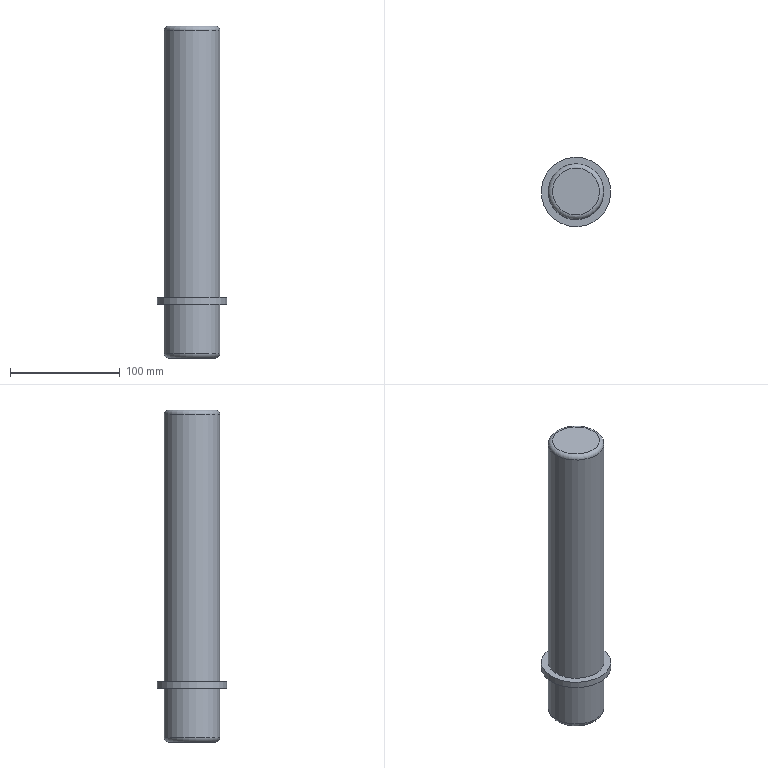Part | STEP file | 1_id1266_x_t | 1 solid | 12 faces | box 63.5 x 63.5 x 303.213 mm | volume 619621 mm3 | cylinder 4 | plane 4 | torus 2 | cone 2 | commonest cylinder face diameters 50.8 x2 4.2 x1 63.5 x1
STEP:
#1=CARTESIAN_POINT('',(0.,0.,0.));
#2=DIRECTION('',(0.,0.,1.));
#3=DIRECTION('',(1.,0.,0.));
#4=AXIS2_PLACEMENT_3D('',#1,#2,#3);
#5=CARTESIAN_POINT('',(-35.188,-151.958,160.));
#6=VERTEX_POINT('',#5);
#7=CARTESIAN_POINT('',(-2.535,-113.042,160.));
#8=VERTEX_POINT('',#7);
#9=CARTESIAN_POINT('',(-18.862,-132.5,160.));
#10=DIRECTION('',(0.,0.,1.));
#11=DIRECTION('',(0.6428,0.766,0.));
#12=AXIS2_PLACEMENT_3D('',#9,#10,#11);
#13=CIRCLE('',#12,25.4);
#14=CARTESIAN_POINT('',(-18.862,-132.5,34.6));
#15=DIRECTION('',(0.,0.,1.));
#16=DIRECTION('',(-0.6428,-0.766,0.));
#17=AXIS2_PLACEMENT_3D('',#14,#15,#16);
#18=CYLINDRICAL_SURFACE('',#17,25.4);
#19=CARTESIAN_POINT('',(-3.142,125.4));
#20=DIRECTION('',(1.,0.));
#21=VECTOR('',#20,1.);
#22=LINE('',#19,#21);
#23=(GEOMETRIC_REPRESENTATION_CONTEXT(2)PARAMETRIC_REPRESENTATION_CONTEXT()REPRESENTATION_CONTEXT('',''));
#24=DEFINITIONAL_REPRESENTATION('',(#22),#23);
#25=PCURVE('',#18,#24);
#26=CARTESIAN_POINT('',(-18.862,-132.5,160.));
#27=DIRECTION('',(0.,0.,1.));
#28=DIRECTION('',(0.6428,0.766,0.));
#29=AXIS2_PLACEMENT_3D('',#26,#27,#28);
#30=TOROIDAL_SURFACE('',#29,21.4,4.);
#31=CARTESIAN_POINT('',(0.,6.283));
#32=DIRECTION('',(1.,0.));
#33=VECTOR('',#32,1.);
#34=LINE('',#31,#33);
#35=(GEOMETRIC_REPRESENTATION_CONTEXT(2)PARAMETRIC_REPRESENTATION_CONTEXT()REPRESENTATION_CONTEXT('',''));
#36=DEFINITIONAL_REPRESENTATION('',(#34),#35);
#37=PCURVE('',#30,#36);
#38=SURFACE_CURVE('',#13,(#25,#37),.PCURVE_S1.);
#39=EDGE_CURVE('',#6,#8,#38,.T.);
#40=ORIENTED_EDGE('',*,*,#39,.F.);
#41=CARTESIAN_POINT('',(-35.188,-151.958,-84.));
#42=VERTEX_POINT('',#41);
#43=CARTESIAN_POINT('',(-35.188,-151.958,-84.));
#44=CARTESIAN_POINT('',(-35.188,-151.958,160.));
#45=B_SPLINE_CURVE_WITH_KNOTS('',1,(#43,#44),.UNSPECIFIED.,.F.,.F.,(2,2),(-118.6,125.4),.PIECEWISE_BEZIER_KNOTS.);
#46=CARTESIAN_POINT('',(0.,0.));
#47=DIRECTION('',(0.,1.));
#48=VECTOR('',#47,1.);
#49=LINE('',#46,#48);
#50=(GEOMETRIC_REPRESENTATION_CONTEXT(2)PARAMETRIC_REPRESENTATION_CONTEXT()REPRESENTATION_CONTEXT('',''));
#51=DEFINITIONAL_REPRESENTATION('',(#49),#50);
#52=PCURVE('',#18,#51);
#53=CARTESIAN_POINT('',(6.283,0.));
#54=DIRECTION('',(0.,1.));
#55=VECTOR('',#54,1.);
#56=LINE('',#53,#55);
#57=(GEOMETRIC_REPRESENTATION_CONTEXT(2)PARAMETRIC_REPRESENTATION_CONTEXT()REPRESENTATION_CONTEXT('',''));
#58=DEFINITIONAL_REPRESENTATION('',(#56),#57);
#59=PCURVE('',#18,#58);
#60=SEAM_CURVE('',#45,(#52,#59),.PCURVE_S1.);
#61=EDGE_CURVE('',#42,#6,#60,.T.);
#62=ORIENTED_EDGE('',*,*,#61,.F.);
#63=CARTESIAN_POINT('',(-18.862,-132.5,-84.));
#64=DIRECTION('',(0.,0.,-1.));
#65=DIRECTION('',(-0.6428,-0.766,0.));
#66=AXIS2_PLACEMENT_3D('',#63,#64,#65);
#67=CIRCLE('',#66,25.4);
#68=CARTESIAN_POINT('',(6.283,-118.6));
#69=DIRECTION('',(-1.,0.));
#70=VECTOR('',#69,1.);
#71=LINE('',#68,#70);
#72=(GEOMETRIC_REPRESENTATION_CONTEXT(2)PARAMETRIC_REPRESENTATION_CONTEXT()REPRESENTATION_CONTEXT('',''));
#73=DEFINITIONAL_REPRESENTATION('',(#71),#72);
#74=PCURVE('',#18,#73);
#75=CARTESIAN_POINT('',(-18.862,-132.5,-84.));
#76=DIRECTION('',(0.,0.,1.));
#77=DIRECTION('',(-0.6428,-0.766,0.));
#78=AXIS2_PLACEMENT_3D('',#75,#76,#77);
#79=PLANE('',#78);
#80=CARTESIAN_POINT('',(25.4,0.));
#81=CARTESIAN_POINT('',(25.4,-43.994));
#82=CARTESIAN_POINT('',(-12.7,-21.997));
#83=CARTESIAN_POINT('',(-50.8,0.));
#84=CARTESIAN_POINT('',(-12.7,21.997));
#85=CARTESIAN_POINT('',(25.4,43.994));
#86=CARTESIAN_POINT('',(25.4,0.));
#87=(BOUNDED_CURVE()B_SPLINE_CURVE(2,(#80,#81,#82,#83,#84,#85,#86),.UNSPECIFIED.,.T.,.F.)B_SPLINE_CURVE_WITH_KNOTS((1,2,2,2,2,1),(-2.094,0.,2.094,4.189,6.283,8.378),.UNSPECIFIED.)CURVE()GEOMETRIC_REPRESENTATION_ITEM()RATIONAL_B_SPLINE_CURVE((1.,0.5,1.,0.5,1.,0.5,1.))REPRESENTATION_ITEM(''));
#88=(GEOMETRIC_REPRESENTATION_CONTEXT(2)PARAMETRIC_REPRESENTATION_CONTEXT()REPRESENTATION_CONTEXT('',''));
#89=DEFINITIONAL_REPRESENTATION('',(#87),#88);
#90=PCURVE('',#79,#89);
#91=SURFACE_CURVE('',#67,(#74,#90),.PCURVE_S1.);
#92=EDGE_CURVE('',#42,#42,#91,.T.);
#93=ORIENTED_EDGE('',*,*,#92,.F.);
#94=ORIENTED_EDGE('',*,*,#61,.T.);
#95=CARTESIAN_POINT('',(-18.862,-132.5,160.));
#96=DIRECTION('',(0.,0.,1.));
#97=DIRECTION('',(0.6428,0.766,0.));
#98=AXIS2_PLACEMENT_3D('',#95,#96,#97);
#99=CIRCLE('',#98,25.4);
#100=CARTESIAN_POINT('',(3.142,125.4));
#101=DIRECTION('',(1.,0.));
#102=VECTOR('',#101,1.);
#103=LINE('',#100,#102);
#104=(GEOMETRIC_REPRESENTATION_CONTEXT(2)PARAMETRIC_REPRESENTATION_CONTEXT()REPRESENTATION_CONTEXT('',''));
#105=DEFINITIONAL_REPRESENTATION('',(#103),#104);
#106=PCURVE('',#18,#105);
#107=CARTESIAN_POINT('',(0.,6.283));
#108=DIRECTION('',(1.,0.));
#109=VECTOR('',#108,1.);
#110=LINE('',#107,#109);
#111=(GEOMETRIC_REPRESENTATION_CONTEXT(2)PARAMETRIC_REPRESENTATION_CONTEXT()REPRESENTATION_CONTEXT('',''));
#112=DEFINITIONAL_REPRESENTATION('',(#110),#111);
#113=PCURVE('',#30,#112);
#114=SURFACE_CURVE('',#99,(#106,#113),.PCURVE_S1.);
#115=EDGE_CURVE('',#8,#6,#114,.T.);
#116=ORIENTED_EDGE('',*,*,#115,.F.);
#117=EDGE_LOOP('',(#40,#62,#93,#94,#116));
#118=FACE_BOUND('',#117,.T.);
#119=ADVANCED_FACE('',(#118),#18,.T.);
#120=CARTESIAN_POINT('',(-39.27,-156.822,-84.));
#121=VERTEX_POINT('',#120);
#122=CARTESIAN_POINT('',(-18.862,-132.5,-84.));
#123=DIRECTION('',(0.,0.,1.));
#124=DIRECTION('',(-0.6428,-0.766,0.));
#125=AXIS2_PLACEMENT_3D('',#122,#123,#124);
#126=CIRCLE('',#125,31.75);
#127=CARTESIAN_POINT('',(0.,0.));
#128=DIRECTION('',(1.,0.));
#129=AXIS2_PLACEMENT_2D('',#127,#128);
#130=CIRCLE('',#129,31.75);
#131=(GEOMETRIC_REPRESENTATION_CONTEXT(2)PARAMETRIC_REPRESENTATION_CONTEXT()REPRESENTATION_CONTEXT('',''));
#132=DEFINITIONAL_REPRESENTATION('',(#130),#131);
#133=PCURVE('',#79,#132);
#134=CARTESIAN_POINT('',(-18.862,-132.5,-84.));
#135=DIRECTION('',(0.,0.,1.));
#136=DIRECTION('',(-0.6428,-0.766,0.));
#137=AXIS2_PLACEMENT_3D('',#134,#135,#136);
#138=CYLINDRICAL_SURFACE('',#137,31.75);
#139=CARTESIAN_POINT('',(0.,0.));
#140=DIRECTION('',(1.,0.));
#141=VECTOR('',#140,1.);
#142=LINE('',#139,#141);
#143=(GEOMETRIC_REPRESENTATION_CONTEXT(2)PARAMETRIC_REPRESENTATION_CONTEXT()REPRESENTATION_CONTEXT('',''));
#144=DEFINITIONAL_REPRESENTATION('',(#142),#143);
#145=PCURVE('',#138,#144);
#146=SURFACE_CURVE('',#126,(#133,#145),.PCURVE_S1.);
#147=EDGE_CURVE('',#121,#121,#146,.T.);
#148=ORIENTED_EDGE('',*,*,#147,.T.);
#149=EDGE_LOOP('',(#148));
#150=FACE_BOUND('',#149,.T.);
#151=ORIENTED_EDGE('',*,*,#92,.T.);
#152=EDGE_LOOP('',(#151));
#153=FACE_BOUND('',#152,.T.);
#154=ADVANCED_FACE('',(#150,#153),#79,.T.);
#155=ORIENTED_EDGE('',*,*,#147,.F.);
#156=CARTESIAN_POINT('',(-39.27,-156.822,-90.));
#157=VERTEX_POINT('',#156);
#158=CARTESIAN_POINT('',(-39.27,-156.822,-90.));
#159=CARTESIAN_POINT('',(-39.27,-156.822,-84.));
#160=B_SPLINE_CURVE_WITH_KNOTS('',1,(#158,#159),.UNSPECIFIED.,.F.,.F.,(2,2),(-6.,0.),.PIECEWISE_BEZIER_KNOTS.);
#161=CARTESIAN_POINT('',(0.,0.));
#162=DIRECTION('',(0.,1.));
#163=VECTOR('',#162,1.);
#164=LINE('',#161,#163);
#165=(GEOMETRIC_REPRESENTATION_CONTEXT(2)PARAMETRIC_REPRESENTATION_CONTEXT()REPRESENTATION_CONTEXT('',''));
#166=DEFINITIONAL_REPRESENTATION('',(#164),#165);
#167=PCURVE('',#138,#166);
#168=CARTESIAN_POINT('',(6.283,0.));
#169=DIRECTION('',(0.,1.));
#170=VECTOR('',#169,1.);
#171=LINE('',#168,#170);
#172=(GEOMETRIC_REPRESENTATION_CONTEXT(2)PARAMETRIC_REPRESENTATION_CONTEXT()REPRESENTATION_CONTEXT('',''));
#173=DEFINITIONAL_REPRESENTATION('',(#171),#172);
#174=PCURVE('',#138,#173);
#175=SEAM_CURVE('',#160,(#167,#174),.PCURVE_S1.);
#176=EDGE_CURVE('',#157,#121,#175,.T.);
#177=ORIENTED_EDGE('',*,*,#176,.F.);
#178=CARTESIAN_POINT('',(1.547,-108.178,-90.));
#179=VERTEX_POINT('',#178);
#180=CARTESIAN_POINT('',(-18.862,-132.5,-90.));
#181=DIRECTION('',(0.,0.,-1.));
#182=DIRECTION('',(0.6428,0.766,0.));
#183=AXIS2_PLACEMENT_3D('',#180,#181,#182);
#184=CIRCLE('',#183,31.75);
#185=CARTESIAN_POINT('',(3.142,-6.));
#186=DIRECTION('',(-1.,0.));
#187=VECTOR('',#186,1.);
#188=LINE('',#185,#187);
#189=(GEOMETRIC_REPRESENTATION_CONTEXT(2)PARAMETRIC_REPRESENTATION_CONTEXT()REPRESENTATION_CONTEXT('',''));
#190=DEFINITIONAL_REPRESENTATION('',(#188),#189);
#191=PCURVE('',#138,#190);
#192=CARTESIAN_POINT('',(-18.862,-132.5,-90.));
#193=DIRECTION('',(0.,0.,1.));
#194=DIRECTION('',(-0.6428,-0.766,0.));
#195=AXIS2_PLACEMENT_3D('',#192,#193,#194);
#196=PLANE('',#195);
#197=CARTESIAN_POINT('',(-31.75,0.));
#198=CARTESIAN_POINT('',(-31.75,54.993));
#199=CARTESIAN_POINT('',(15.875,27.496));
#200=CARTESIAN_POINT('',(63.5,0.));
#201=CARTESIAN_POINT('',(15.875,-27.496));
#202=CARTESIAN_POINT('',(-31.75,-54.993));
#203=CARTESIAN_POINT('',(-31.75,0.));
#204=(BOUNDED_CURVE()B_SPLINE_CURVE(2,(#197,#198,#199,#200,#201,#202,#203),.UNSPECIFIED.,.T.,.F.)B_SPLINE_CURVE_WITH_KNOTS((1,2,2,2,2,1),(-2.094,0.,2.094,4.189,6.283,8.378),.UNSPECIFIED.)CURVE()GEOMETRIC_REPRESENTATION_ITEM()RATIONAL_B_SPLINE_CURVE((1.,0.5,1.,0.5,1.,0.5,1.))REPRESENTATION_ITEM(''));
#205=(GEOMETRIC_REPRESENTATION_CONTEXT(2)PARAMETRIC_REPRESENTATION_CONTEXT()REPRESENTATION_CONTEXT('',''));
#206=DEFINITIONAL_REPRESENTATION('',(#204),#205);
#207=PCURVE('',#196,#206);
#208=SURFACE_CURVE('',#184,(#191,#207),.PCURVE_S1.);
#209=EDGE_CURVE('',#179,#157,#208,.T.);
#210=ORIENTED_EDGE('',*,*,#209,.F.);
#211=CARTESIAN_POINT('',(-18.862,-132.5,-90.));
#212=DIRECTION('',(0.,0.,-1.));
#213=DIRECTION('',(0.6428,0.766,0.));
#214=AXIS2_PLACEMENT_3D('',#211,#212,#213);
#215=CIRCLE('',#214,31.75);
#216=CARTESIAN_POINT('',(9.425,-6.));
#217=DIRECTION('',(-1.,0.));
#218=VECTOR('',#217,1.);
#219=LINE('',#216,#218);
#220=(GEOMETRIC_REPRESENTATION_CONTEXT(2)PARAMETRIC_REPRESENTATION_CONTEXT()REPRESENTATION_CONTEXT('',''));
#221=DEFINITIONAL_REPRESENTATION('',(#219),#220);
#222=PCURVE('',#138,#221);
#223=CARTESIAN_POINT('',(-31.75,0.));
#224=CARTESIAN_POINT('',(-31.75,54.993));
#225=CARTESIAN_POINT('',(15.875,27.496));
#226=CARTESIAN_POINT('',(63.5,0.));
#227=CARTESIAN_POINT('',(15.875,-27.496));
#228=CARTESIAN_POINT('',(-31.75,-54.993));
#229=CARTESIAN_POINT('',(-31.75,0.));
#230=(BOUNDED_CURVE()B_SPLINE_CURVE(2,(#223,#224,#225,#226,#227,#228,#229),.UNSPECIFIED.,.T.,.F.)B_SPLINE_CURVE_WITH_KNOTS((1,2,2,2,2,1),(-2.094,0.,2.094,4.189,6.283,8.378),.UNSPECIFIED.)CURVE()GEOMETRIC_REPRESENTATION_ITEM()RATIONAL_B_SPLINE_CURVE((1.,0.5,1.,0.5,1.,0.5,1.))REPRESENTATION_ITEM(''));
#231=(GEOMETRIC_REPRESENTATION_CONTEXT(2)PARAMETRIC_REPRESENTATION_CONTEXT()REPRESENTATION_CONTEXT('',''));
#232=DEFINITIONAL_REPRESENTATION('',(#230),#231);
#233=PCURVE('',#196,#232);
#234=SURFACE_CURVE('',#215,(#222,#233),.PCURVE_S1.);
#235=EDGE_CURVE('',#157,#179,#234,.T.);
#236=ORIENTED_EDGE('',*,*,#235,.F.);
#237=ORIENTED_EDGE('',*,*,#176,.T.);
#238=EDGE_LOOP('',(#155,#177,#210,#236,#237));
#239=FACE_BOUND('',#238,.T.);
#240=ADVANCED_FACE('',(#239),#138,.T.);
#241=ORIENTED_EDGE('',*,*,#209,.T.);
#242=ORIENTED_EDGE('',*,*,#235,.T.);
#243=EDGE_LOOP('',(#241,#242));
#244=FACE_BOUND('',#243,.T.);
#245=CARTESIAN_POINT('',(-35.188,-151.958,-90.));
#246=VERTEX_POINT('',#245);
#247=CARTESIAN_POINT('',(-2.535,-113.042,-90.));
#248=VERTEX_POINT('',#247);
#249=CARTESIAN_POINT('',(-18.862,-132.5,-90.));
#250=DIRECTION('',(0.,0.,1.));
#251=DIRECTION('',(-0.6428,-0.766,0.));
#252=AXIS2_PLACEMENT_3D('',#249,#250,#251);
#253=CIRCLE('',#252,25.4);
#254=CARTESIAN_POINT('',(0.,0.));
#255=DIRECTION('',(1.,0.));
#256=AXIS2_PLACEMENT_2D('',#254,#255);
#257=CIRCLE('',#256,25.4);
#258=(GEOMETRIC_REPRESENTATION_CONTEXT(2)PARAMETRIC_REPRESENTATION_CONTEXT()REPRESENTATION_CONTEXT('',''));
#259=DEFINITIONAL_REPRESENTATION('',(#257),#258);
#260=PCURVE('',#196,#259);
#261=CARTESIAN_POINT('',(-18.862,-132.5,-135.));
#262=DIRECTION('',(0.,0.,-1.));
#263=DIRECTION('',(0.6428,0.766,0.));
#264=AXIS2_PLACEMENT_3D('',#261,#262,#263);
#265=CYLINDRICAL_SURFACE('',#264,25.4);
#266=CARTESIAN_POINT('',(3.142,-45.));
#267=DIRECTION('',(-1.,0.));
#268=VECTOR('',#267,1.);
#269=LINE('',#266,#268);
#270=(GEOMETRIC_REPRESENTATION_CONTEXT(2)PARAMETRIC_REPRESENTATION_CONTEXT()REPRESENTATION_CONTEXT('',''));
#271=DEFINITIONAL_REPRESENTATION('',(#269),#270);
#272=PCURVE('',#265,#271);
#273=SURFACE_CURVE('',#253,(#260,#272),.PCURVE_S1.);
#274=EDGE_CURVE('',#246,#248,#273,.T.);
#275=ORIENTED_EDGE('',*,*,#274,.T.);
#276=CARTESIAN_POINT('',(-18.862,-132.5,-90.));
#277=DIRECTION('',(0.,0.,1.));
#278=DIRECTION('',(-0.6428,-0.766,0.));
#279=AXIS2_PLACEMENT_3D('',#276,#277,#278);
#280=CIRCLE('',#279,25.4);
#281=CARTESIAN_POINT('',(0.,0.));
#282=DIRECTION('',(1.,0.));
#283=AXIS2_PLACEMENT_2D('',#281,#282);
#284=CIRCLE('',#283,25.4);
#285=(GEOMETRIC_REPRESENTATION_CONTEXT(2)PARAMETRIC_REPRESENTATION_CONTEXT()REPRESENTATION_CONTEXT('',''));
#286=DEFINITIONAL_REPRESENTATION('',(#284),#285);
#287=PCURVE('',#196,#286);
#288=CARTESIAN_POINT('',(9.425,-45.));
#289=DIRECTION('',(-1.,0.));
#290=VECTOR('',#289,1.);
#291=LINE('',#288,#290);
#292=(GEOMETRIC_REPRESENTATION_CONTEXT(2)PARAMETRIC_REPRESENTATION_CONTEXT()REPRESENTATION_CONTEXT('',''));
#293=DEFINITIONAL_REPRESENTATION('',(#291),#292);
#294=PCURVE('',#265,#293);
#295=SURFACE_CURVE('',#280,(#287,#294),.PCURVE_S1.);
#296=EDGE_CURVE('',#248,#246,#295,.T.);
#297=ORIENTED_EDGE('',*,*,#296,.T.);
#298=EDGE_LOOP('',(#275,#297));
#299=FACE_BOUND('',#298,.T.);
#300=ADVANCED_FACE('',(#244,#299),#196,.F.);
#301=CARTESIAN_POINT('',(-2.535,-113.042,-135.212));
#302=VERTEX_POINT('',#301);
#303=CARTESIAN_POINT('',(-18.862,-132.5,-135.212));
#304=DIRECTION('',(0.,0.,-1.));
#305=DIRECTION('',(0.6428,0.766,0.));
#306=AXIS2_PLACEMENT_3D('',#303,#304,#305);
#307=CIRCLE('',#306,25.4);
#308=CARTESIAN_POINT('',(0.,0.2125));
#309=DIRECTION('',(1.,0.));
#310=VECTOR('',#309,1.);
#311=LINE('',#308,#310);
#312=(GEOMETRIC_REPRESENTATION_CONTEXT(2)PARAMETRIC_REPRESENTATION_CONTEXT()REPRESENTATION_CONTEXT('',''));
#313=DEFINITIONAL_REPRESENTATION('',(#311),#312);
#314=PCURVE('',#265,#313);
#315=CARTESIAN_POINT('',(-18.862,-132.5,-135.212));
#316=DIRECTION('',(0.,0.,1.));
#317=DIRECTION('',(0.6428,0.766,0.));
#318=AXIS2_PLACEMENT_3D('',#315,#316,#317);
#319=TOROIDAL_SURFACE('',#318,21.4,4.);
#320=CARTESIAN_POINT('',(6.283,6.283));
#321=DIRECTION('',(-1.,0.));
#322=VECTOR('',#321,1.);
#323=LINE('',#320,#322);
#324=(GEOMETRIC_REPRESENTATION_CONTEXT(2)PARAMETRIC_REPRESENTATION_CONTEXT()REPRESENTATION_CONTEXT('',''));
#325=DEFINITIONAL_REPRESENTATION('',(#323),#324);
#326=PCURVE('',#319,#325);
#327=SURFACE_CURVE('',#307,(#314,#326),.PCURVE_S1.);
#328=EDGE_CURVE('',#302,#302,#327,.T.);
#329=ORIENTED_EDGE('',*,*,#328,.F.);
#330=CARTESIAN_POINT('',(-2.535,-113.042,-90.));
#331=CARTESIAN_POINT('',(-2.535,-113.042,-135.212));
#332=B_SPLINE_CURVE_WITH_KNOTS('',1,(#330,#331),.UNSPECIFIED.,.F.,.F.,(2,2),(-45.,0.2125),.PIECEWISE_BEZIER_KNOTS.);
#333=CARTESIAN_POINT('',(0.,0.));
#334=DIRECTION('',(0.,1.));
#335=VECTOR('',#334,1.);
#336=LINE('',#333,#335);
#337=(GEOMETRIC_REPRESENTATION_CONTEXT(2)PARAMETRIC_REPRESENTATION_CONTEXT()REPRESENTATION_CONTEXT('',''));
#338=DEFINITIONAL_REPRESENTATION('',(#336),#337);
#339=PCURVE('',#265,#338);
#340=CARTESIAN_POINT('',(6.283,0.));
#341=DIRECTION('',(0.,1.));
#342=VECTOR('',#341,1.);
#343=LINE('',#340,#342);
#344=(GEOMETRIC_REPRESENTATION_CONTEXT(2)PARAMETRIC_REPRESENTATION_CONTEXT()REPRESENTATION_CONTEXT('',''));
#345=DEFINITIONAL_REPRESENTATION('',(#343),#344);
#346=PCURVE('',#265,#345);
#347=SEAM_CURVE('',#332,(#339,#346),.PCURVE_S1.);
#348=EDGE_CURVE('',#248,#302,#347,.T.);
#349=ORIENTED_EDGE('',*,*,#348,.F.);
#350=ORIENTED_EDGE('',*,*,#274,.F.);
#351=ORIENTED_EDGE('',*,*,#296,.F.);
#352=ORIENTED_EDGE('',*,*,#348,.T.);
#353=EDGE_LOOP('',(#329,#349,#350,#351,#352));
#354=FACE_BOUND('',#353,.T.);
#355=ADVANCED_FACE('',(#354),#265,.T.);
#356=ORIENTED_EDGE('',*,*,#328,.T.);
#357=CARTESIAN_POINT('',(-5.106,-116.107,-139.212));
#358=VERTEX_POINT('',#357);
#359=CARTESIAN_POINT('',(-5.106,-116.107,-139.212));
#360=CARTESIAN_POINT('',(-4.419,-115.287,-139.212));
#361=CARTESIAN_POINT('',(-3.749,-114.49,-138.872));
#362=CARTESIAN_POINT('',(-3.173,-113.803,-138.22));
#363=CARTESIAN_POINT('',(-2.753,-113.303,-137.323));
#364=CARTESIAN_POINT('',(-2.535,-113.042,-136.282));
#365=CARTESIAN_POINT('',(-2.535,-113.042,-135.212));
#366=(BOUNDED_CURVE()B_SPLINE_CURVE(6,(#359,#360,#361,#362,#363,#364,#365),.UNSPECIFIED.,.F.,.F.)B_SPLINE_CURVE_WITH_KNOTS((7,7),(-1.571,0.),.PIECEWISE_BEZIER_KNOTS.)CURVE()GEOMETRIC_REPRESENTATION_ITEM()RATIONAL_B_SPLINE_CURVE((1.031,1.01,0.9979,0.994,0.9979,1.01,1.031))REPRESENTATION_ITEM(''));
#367=CARTESIAN_POINT('',(0.,6.283));
#368=DIRECTION('',(0.,1.));
#369=VECTOR('',#368,1.);
#370=LINE('',#367,#369);
#371=(GEOMETRIC_REPRESENTATION_CONTEXT(2)PARAMETRIC_REPRESENTATION_CONTEXT()REPRESENTATION_CONTEXT('',''));
#372=DEFINITIONAL_REPRESENTATION('',(#370),#371);
#373=PCURVE('',#319,#372);
#374=CARTESIAN_POINT('',(6.283,6.283));
#375=DIRECTION('',(0.,1.));
#376=VECTOR('',#375,1.);
#377=LINE('',#374,#376);
#378=(GEOMETRIC_REPRESENTATION_CONTEXT(2)PARAMETRIC_REPRESENTATION_CONTEXT()REPRESENTATION_CONTEXT('',''));
#379=DEFINITIONAL_REPRESENTATION('',(#377),#378);
#380=PCURVE('',#319,#379);
#381=SEAM_CURVE('',#366,(#373,#380),.PCURVE_S1.);
#382=EDGE_CURVE('',#358,#302,#381,.T.);
#383=ORIENTED_EDGE('',*,*,#382,.F.);
#384=CARTESIAN_POINT('',(-32.617,-148.893,-139.212));
#385=VERTEX_POINT('',#384);
#386=CARTESIAN_POINT('',(-18.862,-132.5,-139.212));
#387=DIRECTION('',(0.,0.,-1.));
#388=DIRECTION('',(-0.6428,-0.766,0.));
#389=AXIS2_PLACEMENT_3D('',#386,#387,#388);
#390=CIRCLE('',#389,21.4);
#391=CARTESIAN_POINT('',(3.142,4.712));
#392=DIRECTION('',(-1.,0.));
#393=VECTOR('',#392,1.);
#394=LINE('',#391,#393);
#395=(GEOMETRIC_REPRESENTATION_CONTEXT(2)PARAMETRIC_REPRESENTATION_CONTEXT()REPRESENTATION_CONTEXT('',''));
#396=DEFINITIONAL_REPRESENTATION('',(#394),#395);
#397=PCURVE('',#319,#396);
#398=CARTESIAN_POINT('',(-18.862,-132.5,-139.212));
#399=DIRECTION('',(0.,0.,1.));
#400=DIRECTION('',(-0.6428,-0.766,0.));
#401=AXIS2_PLACEMENT_3D('',#398,#399,#400);
#402=PLANE('',#401);
#403=CARTESIAN_POINT('',(21.4,0.));
#404=CARTESIAN_POINT('',(21.4,-37.066));
#405=CARTESIAN_POINT('',(-10.7,-18.533));
#406=CARTESIAN_POINT('',(-42.8,0.));
#407=CARTESIAN_POINT('',(-10.7,18.533));
#408=CARTESIAN_POINT('',(21.4,37.066));
#409=CARTESIAN_POINT('',(21.4,0.));
#410=(BOUNDED_CURVE()B_SPLINE_CURVE(2,(#403,#404,#405,#406,#407,#408,#409),.UNSPECIFIED.,.T.,.F.)B_SPLINE_CURVE_WITH_KNOTS((1,2,2,2,2,1),(-2.094,0.,2.094,4.189,6.283,8.378),.UNSPECIFIED.)CURVE()GEOMETRIC_REPRESENTATION_ITEM()RATIONAL_B_SPLINE_CURVE((1.,0.5,1.,0.5,1.,0.5,1.))REPRESENTATION_ITEM(''));
#411=(GEOMETRIC_REPRESENTATION_CONTEXT(2)PARAMETRIC_REPRESENTATION_CONTEXT()REPRESENTATION_CONTEXT('',''));
#412=DEFINITIONAL_REPRESENTATION('',(#410),#411);
#413=PCURVE('',#402,#412);
#414=SURFACE_CURVE('',#390,(#397,#413),.PCURVE_S1.);
#415=EDGE_CURVE('',#385,#358,#414,.T.);
#416=ORIENTED_EDGE('',*,*,#415,.F.);
#417=CARTESIAN_POINT('',(-18.862,-132.5,-139.212));
#418=DIRECTION('',(0.,0.,-1.));
#419=DIRECTION('',(-0.6428,-0.766,0.));
#420=AXIS2_PLACEMENT_3D('',#417,#418,#419);
#421=CIRCLE('',#420,21.4);
#422=CARTESIAN_POINT('',(9.425,4.712));
#423=DIRECTION('',(-1.,0.));
#424=VECTOR('',#423,1.);
#425=LINE('',#422,#424);
#426=(GEOMETRIC_REPRESENTATION_CONTEXT(2)PARAMETRIC_REPRESENTATION_CONTEXT()REPRESENTATION_CONTEXT('',''));
#427=DEFINITIONAL_REPRESENTATION('',(#425),#426);
#428=PCURVE('',#319,#427);
#429=CARTESIAN_POINT('',(21.4,0.));
#430=CARTESIAN_POINT('',(21.4,-37.066));
#431=CARTESIAN_POINT('',(-10.7,-18.533));
#432=CARTESIAN_POINT('',(-42.8,0.));
#433=CARTESIAN_POINT('',(-10.7,18.533));
#434=CARTESIAN_POINT('',(21.4,37.066));
#435=CARTESIAN_POINT('',(21.4,0.));
#436=(BOUNDED_CURVE()B_SPLINE_CURVE(2,(#429,#430,#431,#432,#433,#434,#435),.UNSPECIFIED.,.T.,.F.)B_SPLINE_CURVE_WITH_KNOTS((1,2,2,2,2,1),(-2.094,0.,2.094,4.189,6.283,8.378),.UNSPECIFIED.)CURVE()GEOMETRIC_REPRESENTATION_ITEM()RATIONAL_B_SPLINE_CURVE((1.,0.5,1.,0.5,1.,0.5,1.))REPRESENTATION_ITEM(''));
#437=(GEOMETRIC_REPRESENTATION_CONTEXT(2)PARAMETRIC_REPRESENTATION_CONTEXT()REPRESENTATION_CONTEXT('',''));
#438=DEFINITIONAL_REPRESENTATION('',(#436),#437);
#439=PCURVE('',#402,#438);
#440=SURFACE_CURVE('',#421,(#428,#439),.PCURVE_S1.);
#441=EDGE_CURVE('',#358,#385,#440,.T.);
#442=ORIENTED_EDGE('',*,*,#441,.F.);
#443=ORIENTED_EDGE('',*,*,#382,.T.);
#444=EDGE_LOOP('',(#356,#383,#416,#442,#443));
#445=FACE_BOUND('',#444,.T.);
#446=ADVANCED_FACE('',(#445),#319,.T.);
#447=ORIENTED_EDGE('',*,*,#415,.T.);
#448=ORIENTED_EDGE('',*,*,#441,.T.);
#449=EDGE_LOOP('',(#447,#448));
#450=FACE_BOUND('',#449,.T.);
#451=CARTESIAN_POINT('',(-23.241,-137.719,-139.212));
#452=VERTEX_POINT('',#451);
#453=CARTESIAN_POINT('',(-18.862,-132.5,-139.212));
#454=DIRECTION('',(0.,0.,1.));
#455=DIRECTION('',(-0.6428,-0.766,0.));
#456=AXIS2_PLACEMENT_3D('',#453,#454,#455);
#457=CIRCLE('',#456,6.812);
#458=CARTESIAN_POINT('',(0.,0.));
#459=DIRECTION('',(1.,0.));
#460=AXIS2_PLACEMENT_2D('',#458,#459);
#461=CIRCLE('',#460,6.812);
#462=(GEOMETRIC_REPRESENTATION_CONTEXT(2)PARAMETRIC_REPRESENTATION_CONTEXT()REPRESENTATION_CONTEXT('',''));
#463=DEFINITIONAL_REPRESENTATION('',(#461),#462);
#464=PCURVE('',#402,#463);
#465=CARTESIAN_POINT('',(-18.862,-132.5,-136.856));
#466=DIRECTION('',(0.,0.,-1.));
#467=DIRECTION('',(-0.6428,-0.766,0.));
#468=AXIS2_PLACEMENT_3D('',#465,#466,#467);
#469=CONICAL_SURFACE('',#468,4.456,0.7854);
#470=CARTESIAN_POINT('',(6.283,2.356));
#471=DIRECTION('',(-1.,0.));
#472=VECTOR('',#471,1.);
#473=LINE('',#470,#472);
#474=(GEOMETRIC_REPRESENTATION_CONTEXT(2)PARAMETRIC_REPRESENTATION_CONTEXT()REPRESENTATION_CONTEXT('',''));
#475=DEFINITIONAL_REPRESENTATION('',(#473),#474);
#476=PCURVE('',#469,#475);
#477=SURFACE_CURVE('',#457,(#464,#476),.PCURVE_S1.);
#478=EDGE_CURVE('',#452,#452,#477,.T.);
#479=ORIENTED_EDGE('',*,*,#478,.T.);
#480=EDGE_LOOP('',(#479));
#481=FACE_BOUND('',#480,.T.);
#482=ADVANCED_FACE('',(#450,#481),#402,.F.);
#483=ORIENTED_EDGE('',*,*,#478,.T.);
#484=CARTESIAN_POINT('',(-20.211,-134.109,-134.5));
#485=VERTEX_POINT('',#484);
#486=CARTESIAN_POINT('',(-20.211,-134.109,-134.5));
#487=CARTESIAN_POINT('',(-23.241,-137.719,-139.213));
#488=B_SPLINE_CURVE_WITH_KNOTS('',1,(#486,#487),.UNSPECIFIED.,.F.,.F.,(2,2),(-3.332,3.332),.PIECEWISE_BEZIER_KNOTS.);
#489=CARTESIAN_POINT('',(0.,0.));
#490=DIRECTION('',(0.,1.));
#491=VECTOR('',#490,1.);
#492=LINE('',#489,#491);
#493=(GEOMETRIC_REPRESENTATION_CONTEXT(2)PARAMETRIC_REPRESENTATION_CONTEXT()REPRESENTATION_CONTEXT('',''));
#494=DEFINITIONAL_REPRESENTATION('',(#492),#493);
#495=PCURVE('',#469,#494);
#496=CARTESIAN_POINT('',(6.283,0.));
#497=DIRECTION('',(0.,1.));
#498=VECTOR('',#497,1.);
#499=LINE('',#496,#498);
#500=(GEOMETRIC_REPRESENTATION_CONTEXT(2)PARAMETRIC_REPRESENTATION_CONTEXT()REPRESENTATION_CONTEXT('',''));
#501=DEFINITIONAL_REPRESENTATION('',(#499),#500);
#502=PCURVE('',#469,#501);
#503=SEAM_CURVE('',#488,(#495,#502),.PCURVE_S1.);
#504=EDGE_CURVE('',#485,#452,#503,.T.);
#505=ORIENTED_EDGE('',*,*,#504,.F.);
#506=CARTESIAN_POINT('',(-18.862,-132.5,-134.5));
#507=DIRECTION('',(0.,0.,1.));
#508=DIRECTION('',(-0.6428,-0.766,0.));
#509=AXIS2_PLACEMENT_3D('',#506,#507,#508);
#510=CIRCLE('',#509,2.1);
#511=CARTESIAN_POINT('',(6.283,-2.356));
#512=DIRECTION('',(-1.,0.));
#513=VECTOR('',#512,1.);
#514=LINE('',#511,#513);
#515=(GEOMETRIC_REPRESENTATION_CONTEXT(2)PARAMETRIC_REPRESENTATION_CONTEXT()REPRESENTATION_CONTEXT('',''));
#516=DEFINITIONAL_REPRESENTATION('',(#514),#515);
#517=PCURVE('',#469,#516);
#518=CARTESIAN_POINT('',(-18.862,-132.5,-106.));
#519=DIRECTION('',(0.,0.,1.));
#520=DIRECTION('',(-0.6428,-0.766,0.));
#521=AXIS2_PLACEMENT_3D('',#518,#519,#520);
#522=CYLINDRICAL_SURFACE('',#521,2.1);
#523=CARTESIAN_POINT('',(0.,-28.5));
#524=DIRECTION('',(1.,0.));
#525=VECTOR('',#524,1.);
#526=LINE('',#523,#525);
#527=(GEOMETRIC_REPRESENTATION_CONTEXT(2)PARAMETRIC_REPRESENTATION_CONTEXT()REPRESENTATION_CONTEXT('',''));
#528=DEFINITIONAL_REPRESENTATION('',(#526),#527);
#529=PCURVE('',#522,#528);
#530=SURFACE_CURVE('',#510,(#517,#529),.PCURVE_S1.);
#531=EDGE_CURVE('',#485,#485,#530,.T.);
#532=ORIENTED_EDGE('',*,*,#531,.F.);
#533=ORIENTED_EDGE('',*,*,#504,.T.);
#534=EDGE_LOOP('',(#483,#505,#532,#533));
#535=FACE_BOUND('',#534,.F.);
#536=ADVANCED_FACE('',(#535),#469,.F.);
#537=CARTESIAN_POINT('',(-20.211,-134.109,-106.));
#538=VERTEX_POINT('',#537);
#539=CARTESIAN_POINT('',(-18.862,-132.5,-106.));
#540=DIRECTION('',(0.,0.,-1.));
#541=DIRECTION('',(-0.6428,-0.766,0.));
#542=AXIS2_PLACEMENT_3D('',#539,#540,#541);
#543=CIRCLE('',#542,2.1);
#544=CARTESIAN_POINT('',(6.283,0.));
#545=DIRECTION('',(-1.,0.));
#546=VECTOR('',#545,1.);
#547=LINE('',#544,#546);
#548=(GEOMETRIC_REPRESENTATION_CONTEXT(2)PARAMETRIC_REPRESENTATION_CONTEXT()REPRESENTATION_CONTEXT('',''));
#549=DEFINITIONAL_REPRESENTATION('',(#547),#548);
#550=PCURVE('',#522,#549);
#551=CARTESIAN_POINT('',(-18.862,-132.5,-105.492));
#552=DIRECTION('',(0.,0.,-1.));
#553=DIRECTION('',(-0.6428,-0.766,0.));
#554=AXIS2_PLACEMENT_3D('',#551,#552,#553);
#555=CONICAL_SURFACE('',#554,1.221,1.047);
#556=CARTESIAN_POINT('',(0.,0.5076));
#557=DIRECTION('',(1.,0.));
#558=VECTOR('',#557,1.);
#559=LINE('',#556,#558);
#560=(GEOMETRIC_REPRESENTATION_CONTEXT(2)PARAMETRIC_REPRESENTATION_CONTEXT()REPRESENTATION_CONTEXT('',''));
#561=DEFINITIONAL_REPRESENTATION('',(#559),#560);
#562=PCURVE('',#555,#561);
#563=SURFACE_CURVE('',#543,(#550,#562),.PCURVE_S1.);
#564=EDGE_CURVE('',#538,#538,#563,.T.);
#565=ORIENTED_EDGE('',*,*,#564,.T.);
#566=CARTESIAN_POINT('',(-20.211,-134.109,-134.5));
#567=CARTESIAN_POINT('',(-20.211,-134.109,-106.));
#568=B_SPLINE_CURVE_WITH_KNOTS('',1,(#566,#567),.UNSPECIFIED.,.F.,.F.,(2,2),(-28.5,0.),.PIECEWISE_BEZIER_KNOTS.);
#569=CARTESIAN_POINT('',(0.,0.));
#570=DIRECTION('',(0.,1.));
#571=VECTOR('',#570,1.);
#572=LINE('',#569,#571);
#573=(GEOMETRIC_REPRESENTATION_CONTEXT(2)PARAMETRIC_REPRESENTATION_CONTEXT()REPRESENTATION_CONTEXT('',''));
#574=DEFINITIONAL_REPRESENTATION('',(#572),#573);
#575=PCURVE('',#522,#574);
#576=CARTESIAN_POINT('',(6.283,0.));
#577=DIRECTION('',(0.,1.));
#578=VECTOR('',#577,1.);
#579=LINE('',#576,#578);
#580=(GEOMETRIC_REPRESENTATION_CONTEXT(2)PARAMETRIC_REPRESENTATION_CONTEXT()REPRESENTATION_CONTEXT('',''));
#581=DEFINITIONAL_REPRESENTATION('',(#579),#580);
#582=PCURVE('',#522,#581);
#583=SEAM_CURVE('',#568,(#575,#582),.PCURVE_S1.);
#584=EDGE_CURVE('',#485,#538,#583,.T.);
#585=ORIENTED_EDGE('',*,*,#584,.F.);
#586=ORIENTED_EDGE('',*,*,#531,.T.);
#587=ORIENTED_EDGE('',*,*,#584,.T.);
#588=EDGE_LOOP('',(#565,#585,#586,#587));
#589=FACE_BOUND('',#588,.F.);
#590=ADVANCED_FACE('',(#589),#522,.F.);
#591=ORIENTED_EDGE('',*,*,#564,.F.);
#592=CARTESIAN_POINT('',(-18.862,-132.5,-104.788));
#593=VERTEX_POINT('',#592);
#594=CARTESIAN_POINT('',(-18.862,-132.5,-104.788));
#595=CARTESIAN_POINT('',(-20.211,-134.109,-106.));
#596=B_SPLINE_CURVE_WITH_KNOTS('',1,(#594,#595),.UNSPECIFIED.,.F.,.F.,(2,2),(-1.41,1.015),.PIECEWISE_BEZIER_KNOTS.);
#597=CARTESIAN_POINT('',(0.,0.));
#598=DIRECTION('',(0.,1.));
#599=VECTOR('',#598,1.);
#600=LINE('',#597,#599);
#601=(GEOMETRIC_REPRESENTATION_CONTEXT(2)PARAMETRIC_REPRESENTATION_CONTEXT()REPRESENTATION_CONTEXT('',''));
#602=DEFINITIONAL_REPRESENTATION('',(#600),#601);
#603=PCURVE('',#555,#602);
#604=CARTESIAN_POINT('',(6.283,0.));
#605=DIRECTION('',(0.,1.));
#606=VECTOR('',#605,1.);
#607=LINE('',#604,#606);
#608=(GEOMETRIC_REPRESENTATION_CONTEXT(2)PARAMETRIC_REPRESENTATION_CONTEXT()REPRESENTATION_CONTEXT('',''));
#609=DEFINITIONAL_REPRESENTATION('',(#607),#608);
#610=PCURVE('',#555,#609);
#611=SEAM_CURVE('',#596,(#603,#610),.PCURVE_S1.);
#612=EDGE_CURVE('',#593,#538,#611,.T.);
#613=ORIENTED_EDGE('',*,*,#612,.F.);
#614=ORIENTED_EDGE('',*,*,#612,.T.);
#615=EDGE_LOOP('',(#591,#613,#614));
#616=FACE_BOUND('',#615,.F.);
#617=ADVANCED_FACE('',(#616),#555,.F.);
#618=CARTESIAN_POINT('',(-5.106,-116.107,164.));
#619=VERTEX_POINT('',#618);
#620=CARTESIAN_POINT('',(-18.862,-132.5,164.));
#621=DIRECTION('',(0.,0.,1.));
#622=DIRECTION('',(0.6428,0.766,0.));
#623=AXIS2_PLACEMENT_3D('',#620,#621,#622);
#624=CIRCLE('',#623,21.4);
#625=CARTESIAN_POINT('',(0.,7.854));
#626=DIRECTION('',(1.,0.));
#627=VECTOR('',#626,1.);
#628=LINE('',#625,#627);
#629=(GEOMETRIC_REPRESENTATION_CONTEXT(2)PARAMETRIC_REPRESENTATION_CONTEXT()REPRESENTATION_CONTEXT('',''));
#630=DEFINITIONAL_REPRESENTATION('',(#628),#629);
#631=PCURVE('',#30,#630);
#632=CARTESIAN_POINT('',(-18.862,-132.5,164.));
#633=DIRECTION('',(0.,0.,1.));
#634=DIRECTION('',(-0.6428,-0.766,0.));
#635=AXIS2_PLACEMENT_3D('',#632,#633,#634);
#636=PLANE('',#635);
#637=CARTESIAN_POINT('',(0.,0.));
#638=DIRECTION('',(-1.,0.));
#639=AXIS2_PLACEMENT_2D('',#637,#638);
#640=CIRCLE('',#639,21.4);
#641=(GEOMETRIC_REPRESENTATION_CONTEXT(2)PARAMETRIC_REPRESENTATION_CONTEXT()REPRESENTATION_CONTEXT('',''));
#642=DEFINITIONAL_REPRESENTATION('',(#640),#641);
#643=PCURVE('',#636,#642);
#644=SURFACE_CURVE('',#624,(#631,#643),.PCURVE_S1.);
#645=EDGE_CURVE('',#619,#619,#644,.T.);
#646=ORIENTED_EDGE('',*,*,#645,.F.);
#647=CARTESIAN_POINT('',(-2.535,-113.042,160.));
#648=CARTESIAN_POINT('',(-2.535,-113.042,161.069));
#649=CARTESIAN_POINT('',(-2.753,-113.303,162.111));
#650=CARTESIAN_POINT('',(-3.173,-113.803,163.008));
#651=CARTESIAN_POINT('',(-3.749,-114.49,163.66));
#652=CARTESIAN_POINT('',(-4.419,-115.287,164.));
#653=CARTESIAN_POINT('',(-5.106,-116.107,164.));
#654=(BOUNDED_CURVE()B_SPLINE_CURVE(6,(#647,#648,#649,#650,#651,#652,#653),.UNSPECIFIED.,.F.,.F.)B_SPLINE_CURVE_WITH_KNOTS((7,7),(0.,1.571),.PIECEWISE_BEZIER_KNOTS.)CURVE()GEOMETRIC_REPRESENTATION_ITEM()RATIONAL_B_SPLINE_CURVE((1.031,1.01,0.9979,0.994,0.9979,1.01,1.031))REPRESENTATION_ITEM(''));
#655=CARTESIAN_POINT('',(0.,6.283));
#656=DIRECTION('',(0.,1.));
#657=VECTOR('',#656,1.);
#658=LINE('',#655,#657);
#659=(GEOMETRIC_REPRESENTATION_CONTEXT(2)PARAMETRIC_REPRESENTATION_CONTEXT()REPRESENTATION_CONTEXT('',''));
#660=DEFINITIONAL_REPRESENTATION('',(#658),#659);
#661=PCURVE('',#30,#660);
#662=CARTESIAN_POINT('',(6.283,6.283));
#663=DIRECTION('',(0.,1.));
#664=VECTOR('',#663,1.);
#665=LINE('',#662,#664);
#666=(GEOMETRIC_REPRESENTATION_CONTEXT(2)PARAMETRIC_REPRESENTATION_CONTEXT()REPRESENTATION_CONTEXT('',''));
#667=DEFINITIONAL_REPRESENTATION('',(#665),#666);
#668=PCURVE('',#30,#667);
#669=SEAM_CURVE('',#654,(#661,#668),.PCURVE_S1.);
#670=EDGE_CURVE('',#8,#619,#669,.T.);
#671=ORIENTED_EDGE('',*,*,#670,.F.);
#672=ORIENTED_EDGE('',*,*,#115,.T.);
#673=ORIENTED_EDGE('',*,*,#39,.T.);
#674=ORIENTED_EDGE('',*,*,#670,.T.);
#675=EDGE_LOOP('',(#646,#671,#672,#673,#674));
#676=FACE_BOUND('',#675,.T.);
#677=ADVANCED_FACE('',(#676),#30,.T.);
#678=ORIENTED_EDGE('',*,*,#645,.T.);
#679=EDGE_LOOP('',(#678));
#680=FACE_BOUND('',#679,.T.);
#681=ADVANCED_FACE('',(#680),#636,.T.);
#682=CLOSED_SHELL('',(#119,#154,#240,#300,#355,#446,#482,#536,#590,#617,#677,#681));
#683=MANIFOLD_SOLID_BREP('',#682);
#684=(LENGTH_UNIT()NAMED_UNIT(*)SI_UNIT(.MILLI.,.METRE.));
#685=UNCERTAINTY_MEASURE_WITH_UNIT(LENGTH_MEASURE(0.000005),#684,'','');
#686=(NAMED_UNIT(*)PLANE_ANGLE_UNIT()SI_UNIT($,.RADIAN.));
#687=(NAMED_UNIT(*)SI_UNIT($,.STERADIAN.)SOLID_ANGLE_UNIT());
#688=(GEOMETRIC_REPRESENTATION_CONTEXT(3)GLOBAL_UNCERTAINTY_ASSIGNED_CONTEXT((#685))GLOBAL_UNIT_ASSIGNED_CONTEXT((#684,#686,#687))REPRESENTATION_CONTEXT('',''));
#689=ADVANCED_BREP_SHAPE_REPRESENTATION('',(#4,#683),#688);